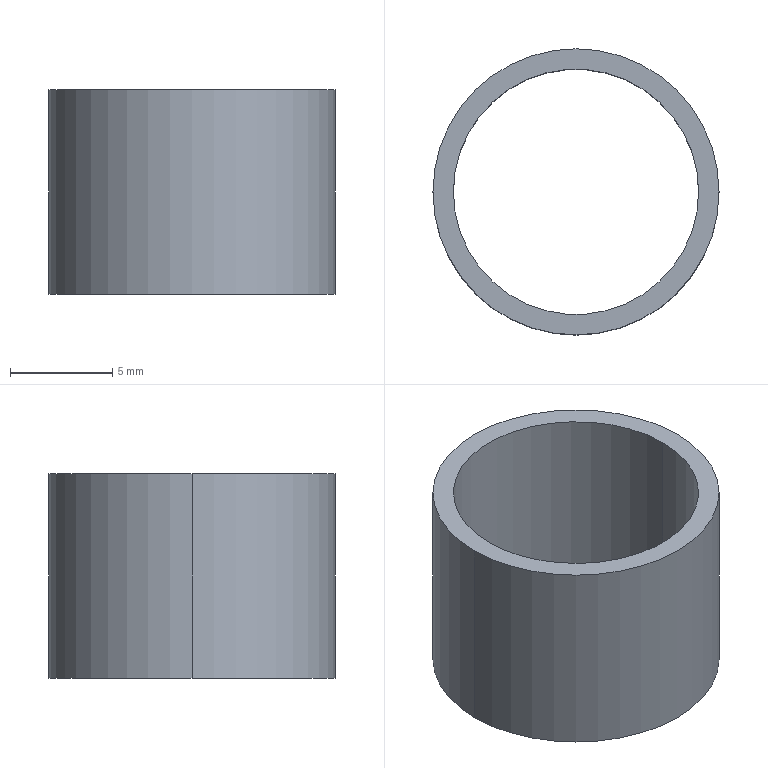Part | STEP file | steel sleeve 12-14-10 | 1 solid | 6 faces | box 14 x 14 x 10 mm | volume 408.407 mm3 | cylinder 4 | plane 2 | commonest cylinder face diameters 12 x2 14 x2
STEP:
#1=CARTESIAN_POINT('',(0.,0.,0.));
#2=DIRECTION('',(0.,0.,1.));
#3=DIRECTION('',(1.,0.,0.));
#4=AXIS2_PLACEMENT_3D('',#1,#2,#3);
#5=CARTESIAN_POINT('',(-6.,0.,10.));
#6=VERTEX_POINT('',#5);
#7=CARTESIAN_POINT('',(-6.,0.,0.));
#8=VERTEX_POINT('',#7);
#9=CARTESIAN_POINT('',(-6.,0.,10.));
#10=DIRECTION('',(0.,0.,-1.));
#11=VECTOR('',#10,1.);
#12=LINE('',#9,#11);
#13=CARTESIAN_POINT('',(0.,0.,10.));
#14=DIRECTION('',(0.,0.,-1.));
#15=DIRECTION('',(-1.,0.,0.));
#16=AXIS2_PLACEMENT_3D('',#13,#14,#15);
#17=CYLINDRICAL_SURFACE('',#16,6.);
#18=CARTESIAN_POINT('',(6.283,0.));
#19=DIRECTION('',(0.,1.));
#20=VECTOR('',#19,1.);
#21=LINE('',#18,#20);
#22=(GEOMETRIC_REPRESENTATION_CONTEXT(2)PARAMETRIC_REPRESENTATION_CONTEXT()REPRESENTATION_CONTEXT('',''));
#23=DEFINITIONAL_REPRESENTATION('',(#21),#22);
#24=PCURVE('',#17,#23);
#25=CARTESIAN_POINT('',(0.,0.,10.));
#26=DIRECTION('',(0.,0.,-1.));
#27=DIRECTION('',(-1.,0.,0.));
#28=AXIS2_PLACEMENT_3D('',#25,#26,#27);
#29=CYLINDRICAL_SURFACE('',#28,6.);
#30=CARTESIAN_POINT('',(0.,0.));
#31=DIRECTION('',(0.,1.));
#32=VECTOR('',#31,1.);
#33=LINE('',#30,#32);
#34=(GEOMETRIC_REPRESENTATION_CONTEXT(2)PARAMETRIC_REPRESENTATION_CONTEXT()REPRESENTATION_CONTEXT('',''));
#35=DEFINITIONAL_REPRESENTATION('',(#33),#34);
#36=PCURVE('',#29,#35);
#37=SURFACE_CURVE('',#12,(#24,#36),.PCURVE_S1.);
#38=EDGE_CURVE('',#6,#8,#37,.T.);
#39=ORIENTED_EDGE('',*,*,#38,.T.);
#40=CARTESIAN_POINT('',(6.,0.,0.));
#41=VERTEX_POINT('',#40);
#42=CARTESIAN_POINT('',(0.,0.,0.));
#43=DIRECTION('',(0.,0.,1.));
#44=DIRECTION('',(1.,0.,0.));
#45=AXIS2_PLACEMENT_3D('',#42,#43,#44);
#46=CIRCLE('',#45,6.);
#47=CARTESIAN_POINT('',(9.425,10.));
#48=DIRECTION('',(-1.,0.));
#49=VECTOR('',#48,1.);
#50=LINE('',#47,#49);
#51=(GEOMETRIC_REPRESENTATION_CONTEXT(2)PARAMETRIC_REPRESENTATION_CONTEXT()REPRESENTATION_CONTEXT('',''));
#52=DEFINITIONAL_REPRESENTATION('',(#50),#51);
#53=PCURVE('',#17,#52);
#54=CARTESIAN_POINT('',(0.,0.,0.));
#55=DIRECTION('',(0.,0.,1.));
#56=DIRECTION('',(1.,0.,0.));
#57=AXIS2_PLACEMENT_3D('',#54,#55,#56);
#58=PLANE('',#57);
#59=CARTESIAN_POINT('',(0.,0.));
#60=DIRECTION('',(1.,0.));
#61=AXIS2_PLACEMENT_2D('',#59,#60);
#62=CIRCLE('',#61,6.);
#63=(GEOMETRIC_REPRESENTATION_CONTEXT(2)PARAMETRIC_REPRESENTATION_CONTEXT()REPRESENTATION_CONTEXT('',''));
#64=DEFINITIONAL_REPRESENTATION('',(#62),#63);
#65=PCURVE('',#58,#64);
#66=SURFACE_CURVE('',#46,(#53,#65),.PCURVE_S1.);
#67=EDGE_CURVE('',#8,#41,#66,.T.);
#68=ORIENTED_EDGE('',*,*,#67,.T.);
#69=CARTESIAN_POINT('',(6.,0.,10.));
#70=VERTEX_POINT('',#69);
#71=CARTESIAN_POINT('',(6.,0.,10.));
#72=DIRECTION('',(0.,0.,-1.));
#73=VECTOR('',#72,1.);
#74=LINE('',#71,#73);
#75=CARTESIAN_POINT('',(3.142,0.));
#76=DIRECTION('',(0.,1.));
#77=VECTOR('',#76,1.);
#78=LINE('',#75,#77);
#79=(GEOMETRIC_REPRESENTATION_CONTEXT(2)PARAMETRIC_REPRESENTATION_CONTEXT()REPRESENTATION_CONTEXT('',''));
#80=DEFINITIONAL_REPRESENTATION('',(#78),#79);
#81=PCURVE('',#17,#80);
#82=CARTESIAN_POINT('',(3.142,0.));
#83=DIRECTION('',(0.,1.));
#84=VECTOR('',#83,1.);
#85=LINE('',#82,#84);
#86=(GEOMETRIC_REPRESENTATION_CONTEXT(2)PARAMETRIC_REPRESENTATION_CONTEXT()REPRESENTATION_CONTEXT('',''));
#87=DEFINITIONAL_REPRESENTATION('',(#85),#86);
#88=PCURVE('',#29,#87);
#89=SURFACE_CURVE('',#74,(#81,#88),.PCURVE_S1.);
#90=EDGE_CURVE('',#70,#41,#89,.T.);
#91=ORIENTED_EDGE('',*,*,#90,.F.);
#92=CARTESIAN_POINT('',(0.,0.,10.));
#93=DIRECTION('',(0.,0.,1.));
#94=DIRECTION('',(1.,0.,0.));
#95=AXIS2_PLACEMENT_3D('',#92,#93,#94);
#96=CIRCLE('',#95,6.);
#97=CARTESIAN_POINT('',(9.425,0.));
#98=DIRECTION('',(-1.,0.));
#99=VECTOR('',#98,1.);
#100=LINE('',#97,#99);
#101=(GEOMETRIC_REPRESENTATION_CONTEXT(2)PARAMETRIC_REPRESENTATION_CONTEXT()REPRESENTATION_CONTEXT('',''));
#102=DEFINITIONAL_REPRESENTATION('',(#100),#101);
#103=PCURVE('',#17,#102);
#104=CARTESIAN_POINT('',(0.,0.,10.));
#105=DIRECTION('',(0.,0.,1.));
#106=DIRECTION('',(1.,0.,0.));
#107=AXIS2_PLACEMENT_3D('',#104,#105,#106);
#108=PLANE('',#107);
#109=CARTESIAN_POINT('',(0.,0.));
#110=DIRECTION('',(1.,0.));
#111=AXIS2_PLACEMENT_2D('',#109,#110);
#112=CIRCLE('',#111,6.);
#113=(GEOMETRIC_REPRESENTATION_CONTEXT(2)PARAMETRIC_REPRESENTATION_CONTEXT()REPRESENTATION_CONTEXT('',''));
#114=DEFINITIONAL_REPRESENTATION('',(#112),#113);
#115=PCURVE('',#108,#114);
#116=SURFACE_CURVE('',#96,(#103,#115),.PCURVE_S1.);
#117=EDGE_CURVE('',#6,#70,#116,.T.);
#118=ORIENTED_EDGE('',*,*,#117,.F.);
#119=EDGE_LOOP('',(#39,#68,#91,#118));
#120=FACE_BOUND('',#119,.F.);
#121=ADVANCED_FACE('',(#120),#17,.F.);
#122=CARTESIAN_POINT('',(7.,0.,10.));
#123=VERTEX_POINT('',#122);
#124=CARTESIAN_POINT('',(-7.,0.,10.));
#125=VERTEX_POINT('',#124);
#126=CARTESIAN_POINT('',(0.,0.,10.));
#127=DIRECTION('',(0.,0.,1.));
#128=DIRECTION('',(1.,0.,0.));
#129=AXIS2_PLACEMENT_3D('',#126,#127,#128);
#130=CIRCLE('',#129,7.);
#131=CARTESIAN_POINT('',(0.,0.,10.));
#132=DIRECTION('',(0.,0.,-1.));
#133=DIRECTION('',(-1.,0.,0.));
#134=AXIS2_PLACEMENT_3D('',#131,#132,#133);
#135=CYLINDRICAL_SURFACE('',#134,7.);
#136=CARTESIAN_POINT('',(3.142,0.));
#137=DIRECTION('',(-1.,0.));
#138=VECTOR('',#137,1.);
#139=LINE('',#136,#138);
#140=(GEOMETRIC_REPRESENTATION_CONTEXT(2)PARAMETRIC_REPRESENTATION_CONTEXT()REPRESENTATION_CONTEXT('',''));
#141=DEFINITIONAL_REPRESENTATION('',(#139),#140);
#142=PCURVE('',#135,#141);
#143=CARTESIAN_POINT('',(0.,0.));
#144=DIRECTION('',(1.,0.));
#145=AXIS2_PLACEMENT_2D('',#143,#144);
#146=CIRCLE('',#145,7.);
#147=(GEOMETRIC_REPRESENTATION_CONTEXT(2)PARAMETRIC_REPRESENTATION_CONTEXT()REPRESENTATION_CONTEXT('',''));
#148=DEFINITIONAL_REPRESENTATION('',(#146),#147);
#149=PCURVE('',#108,#148);
#150=SURFACE_CURVE('',#130,(#142,#149),.PCURVE_S1.);
#151=EDGE_CURVE('',#123,#125,#150,.T.);
#152=ORIENTED_EDGE('',*,*,#151,.F.);
#153=CARTESIAN_POINT('',(7.,0.,0.));
#154=VERTEX_POINT('',#153);
#155=CARTESIAN_POINT('',(7.,0.,10.));
#156=DIRECTION('',(0.,0.,-1.));
#157=VECTOR('',#156,1.);
#158=LINE('',#155,#157);
#159=CARTESIAN_POINT('',(3.142,0.));
#160=DIRECTION('',(0.,1.));
#161=VECTOR('',#160,1.);
#162=LINE('',#159,#161);
#163=(GEOMETRIC_REPRESENTATION_CONTEXT(2)PARAMETRIC_REPRESENTATION_CONTEXT()REPRESENTATION_CONTEXT('',''));
#164=DEFINITIONAL_REPRESENTATION('',(#162),#163);
#165=PCURVE('',#135,#164);
#166=CARTESIAN_POINT('',(0.,0.,10.));
#167=DIRECTION('',(0.,0.,-1.));
#168=DIRECTION('',(-1.,0.,0.));
#169=AXIS2_PLACEMENT_3D('',#166,#167,#168);
#170=CYLINDRICAL_SURFACE('',#169,7.);
#171=CARTESIAN_POINT('',(3.142,0.));
#172=DIRECTION('',(0.,1.));
#173=VECTOR('',#172,1.);
#174=LINE('',#171,#173);
#175=(GEOMETRIC_REPRESENTATION_CONTEXT(2)PARAMETRIC_REPRESENTATION_CONTEXT()REPRESENTATION_CONTEXT('',''));
#176=DEFINITIONAL_REPRESENTATION('',(#174),#175);
#177=PCURVE('',#170,#176);
#178=SURFACE_CURVE('',#158,(#165,#177),.PCURVE_S1.);
#179=EDGE_CURVE('',#123,#154,#178,.T.);
#180=ORIENTED_EDGE('',*,*,#179,.T.);
#181=CARTESIAN_POINT('',(-7.,0.,0.));
#182=VERTEX_POINT('',#181);
#183=CARTESIAN_POINT('',(0.,0.,0.));
#184=DIRECTION('',(0.,0.,1.));
#185=DIRECTION('',(1.,0.,0.));
#186=AXIS2_PLACEMENT_3D('',#183,#184,#185);
#187=CIRCLE('',#186,7.);
#188=CARTESIAN_POINT('',(3.142,10.));
#189=DIRECTION('',(-1.,0.));
#190=VECTOR('',#189,1.);
#191=LINE('',#188,#190);
#192=(GEOMETRIC_REPRESENTATION_CONTEXT(2)PARAMETRIC_REPRESENTATION_CONTEXT()REPRESENTATION_CONTEXT('',''));
#193=DEFINITIONAL_REPRESENTATION('',(#191),#192);
#194=PCURVE('',#135,#193);
#195=CARTESIAN_POINT('',(0.,0.));
#196=DIRECTION('',(1.,0.));
#197=AXIS2_PLACEMENT_2D('',#195,#196);
#198=CIRCLE('',#197,7.);
#199=(GEOMETRIC_REPRESENTATION_CONTEXT(2)PARAMETRIC_REPRESENTATION_CONTEXT()REPRESENTATION_CONTEXT('',''));
#200=DEFINITIONAL_REPRESENTATION('',(#198),#199);
#201=PCURVE('',#58,#200);
#202=SURFACE_CURVE('',#187,(#194,#201),.PCURVE_S1.);
#203=EDGE_CURVE('',#154,#182,#202,.T.);
#204=ORIENTED_EDGE('',*,*,#203,.T.);
#205=CARTESIAN_POINT('',(-7.,0.,10.));
#206=DIRECTION('',(0.,0.,-1.));
#207=VECTOR('',#206,1.);
#208=LINE('',#205,#207);
#209=CARTESIAN_POINT('',(0.,0.));
#210=DIRECTION('',(0.,1.));
#211=VECTOR('',#210,1.);
#212=LINE('',#209,#211);
#213=(GEOMETRIC_REPRESENTATION_CONTEXT(2)PARAMETRIC_REPRESENTATION_CONTEXT()REPRESENTATION_CONTEXT('',''));
#214=DEFINITIONAL_REPRESENTATION('',(#212),#213);
#215=PCURVE('',#135,#214);
#216=CARTESIAN_POINT('',(6.283,0.));
#217=DIRECTION('',(0.,1.));
#218=VECTOR('',#217,1.);
#219=LINE('',#216,#218);
#220=(GEOMETRIC_REPRESENTATION_CONTEXT(2)PARAMETRIC_REPRESENTATION_CONTEXT()REPRESENTATION_CONTEXT('',''));
#221=DEFINITIONAL_REPRESENTATION('',(#219),#220);
#222=PCURVE('',#170,#221);
#223=SURFACE_CURVE('',#208,(#215,#222),.PCURVE_S1.);
#224=EDGE_CURVE('',#125,#182,#223,.T.);
#225=ORIENTED_EDGE('',*,*,#224,.F.);
#226=EDGE_LOOP('',(#152,#180,#204,#225));
#227=FACE_BOUND('',#226,.T.);
#228=ADVANCED_FACE('',(#227),#135,.T.);
#229=CARTESIAN_POINT('',(0.,0.,10.));
#230=DIRECTION('',(0.,0.,1.));
#231=DIRECTION('',(1.,0.,0.));
#232=AXIS2_PLACEMENT_3D('',#229,#230,#231);
#233=CIRCLE('',#232,7.);
#234=CARTESIAN_POINT('',(0.,0.));
#235=DIRECTION('',(1.,0.));
#236=AXIS2_PLACEMENT_2D('',#234,#235);
#237=CIRCLE('',#236,7.);
#238=(GEOMETRIC_REPRESENTATION_CONTEXT(2)PARAMETRIC_REPRESENTATION_CONTEXT()REPRESENTATION_CONTEXT('',''));
#239=DEFINITIONAL_REPRESENTATION('',(#237),#238);
#240=PCURVE('',#108,#239);
#241=CARTESIAN_POINT('',(9.425,0.));
#242=DIRECTION('',(-1.,0.));
#243=VECTOR('',#242,1.);
#244=LINE('',#241,#243);
#245=(GEOMETRIC_REPRESENTATION_CONTEXT(2)PARAMETRIC_REPRESENTATION_CONTEXT()REPRESENTATION_CONTEXT('',''));
#246=DEFINITIONAL_REPRESENTATION('',(#244),#245);
#247=PCURVE('',#170,#246);
#248=SURFACE_CURVE('',#233,(#240,#247),.PCURVE_S1.);
#249=EDGE_CURVE('',#125,#123,#248,.T.);
#250=ORIENTED_EDGE('',*,*,#249,.T.);
#251=ORIENTED_EDGE('',*,*,#151,.T.);
#252=EDGE_LOOP('',(#250,#251));
#253=FACE_BOUND('',#252,.T.);
#254=ORIENTED_EDGE('',*,*,#117,.F.);
#255=CARTESIAN_POINT('',(0.,0.,10.));
#256=DIRECTION('',(0.,0.,1.));
#257=DIRECTION('',(1.,0.,0.));
#258=AXIS2_PLACEMENT_3D('',#255,#256,#257);
#259=CIRCLE('',#258,6.);
#260=CARTESIAN_POINT('',(0.,0.));
#261=DIRECTION('',(1.,0.));
#262=AXIS2_PLACEMENT_2D('',#260,#261);
#263=CIRCLE('',#262,6.);
#264=(GEOMETRIC_REPRESENTATION_CONTEXT(2)PARAMETRIC_REPRESENTATION_CONTEXT()REPRESENTATION_CONTEXT('',''));
#265=DEFINITIONAL_REPRESENTATION('',(#263),#264);
#266=PCURVE('',#108,#265);
#267=CARTESIAN_POINT('',(3.142,0.));
#268=DIRECTION('',(-1.,0.));
#269=VECTOR('',#268,1.);
#270=LINE('',#267,#269);
#271=(GEOMETRIC_REPRESENTATION_CONTEXT(2)PARAMETRIC_REPRESENTATION_CONTEXT()REPRESENTATION_CONTEXT('',''));
#272=DEFINITIONAL_REPRESENTATION('',(#270),#271);
#273=PCURVE('',#29,#272);
#274=SURFACE_CURVE('',#259,(#266,#273),.PCURVE_S1.);
#275=EDGE_CURVE('',#70,#6,#274,.T.);
#276=ORIENTED_EDGE('',*,*,#275,.F.);
#277=EDGE_LOOP('',(#254,#276));
#278=FACE_BOUND('',#277,.T.);
#279=ADVANCED_FACE('',(#253,#278),#108,.T.);
#280=CARTESIAN_POINT('',(0.,0.,0.));
#281=DIRECTION('',(0.,0.,1.));
#282=DIRECTION('',(1.,0.,0.));
#283=AXIS2_PLACEMENT_3D('',#280,#281,#282);
#284=CIRCLE('',#283,7.);
#285=CARTESIAN_POINT('',(0.,0.));
#286=DIRECTION('',(1.,0.));
#287=AXIS2_PLACEMENT_2D('',#285,#286);
#288=CIRCLE('',#287,7.);
#289=(GEOMETRIC_REPRESENTATION_CONTEXT(2)PARAMETRIC_REPRESENTATION_CONTEXT()REPRESENTATION_CONTEXT('',''));
#290=DEFINITIONAL_REPRESENTATION('',(#288),#289);
#291=PCURVE('',#58,#290);
#292=CARTESIAN_POINT('',(9.425,10.));
#293=DIRECTION('',(-1.,0.));
#294=VECTOR('',#293,1.);
#295=LINE('',#292,#294);
#296=(GEOMETRIC_REPRESENTATION_CONTEXT(2)PARAMETRIC_REPRESENTATION_CONTEXT()REPRESENTATION_CONTEXT('',''));
#297=DEFINITIONAL_REPRESENTATION('',(#295),#296);
#298=PCURVE('',#170,#297);
#299=SURFACE_CURVE('',#284,(#291,#298),.PCURVE_S1.);
#300=EDGE_CURVE('',#182,#154,#299,.T.);
#301=ORIENTED_EDGE('',*,*,#300,.F.);
#302=ORIENTED_EDGE('',*,*,#203,.F.);
#303=EDGE_LOOP('',(#301,#302));
#304=FACE_BOUND('',#303,.T.);
#305=ORIENTED_EDGE('',*,*,#67,.T.);
#306=CARTESIAN_POINT('',(0.,0.,0.));
#307=DIRECTION('',(0.,0.,1.));
#308=DIRECTION('',(1.,0.,0.));
#309=AXIS2_PLACEMENT_3D('',#306,#307,#308);
#310=CIRCLE('',#309,6.);
#311=CARTESIAN_POINT('',(0.,0.));
#312=DIRECTION('',(1.,0.));
#313=AXIS2_PLACEMENT_2D('',#311,#312);
#314=CIRCLE('',#313,6.);
#315=(GEOMETRIC_REPRESENTATION_CONTEXT(2)PARAMETRIC_REPRESENTATION_CONTEXT()REPRESENTATION_CONTEXT('',''));
#316=DEFINITIONAL_REPRESENTATION('',(#314),#315);
#317=PCURVE('',#58,#316);
#318=CARTESIAN_POINT('',(3.142,10.));
#319=DIRECTION('',(-1.,0.));
#320=VECTOR('',#319,1.);
#321=LINE('',#318,#320);
#322=(GEOMETRIC_REPRESENTATION_CONTEXT(2)PARAMETRIC_REPRESENTATION_CONTEXT()REPRESENTATION_CONTEXT('',''));
#323=DEFINITIONAL_REPRESENTATION('',(#321),#322);
#324=PCURVE('',#29,#323);
#325=SURFACE_CURVE('',#310,(#317,#324),.PCURVE_S1.);
#326=EDGE_CURVE('',#41,#8,#325,.T.);
#327=ORIENTED_EDGE('',*,*,#326,.T.);
#328=EDGE_LOOP('',(#305,#327));
#329=FACE_BOUND('',#328,.T.);
#330=ADVANCED_FACE('',(#304,#329),#58,.F.);
#331=ORIENTED_EDGE('',*,*,#179,.F.);
#332=ORIENTED_EDGE('',*,*,#249,.F.);
#333=ORIENTED_EDGE('',*,*,#224,.T.);
#334=ORIENTED_EDGE('',*,*,#300,.T.);
#335=EDGE_LOOP('',(#331,#332,#333,#334));
#336=FACE_BOUND('',#335,.T.);
#337=ADVANCED_FACE('',(#336),#170,.T.);
#338=ORIENTED_EDGE('',*,*,#326,.T.);
#339=ORIENTED_EDGE('',*,*,#38,.F.);
#340=ORIENTED_EDGE('',*,*,#275,.F.);
#341=ORIENTED_EDGE('',*,*,#90,.T.);
#342=EDGE_LOOP('',(#338,#339,#340,#341));
#343=FACE_BOUND('',#342,.F.);
#344=ADVANCED_FACE('',(#343),#29,.F.);
#345=CLOSED_SHELL('',(#121,#228,#279,#330,#337,#344));
#346=MANIFOLD_SOLID_BREP('',#345);
#347=(LENGTH_UNIT()NAMED_UNIT(*)SI_UNIT(.MILLI.,.METRE.));
#348=UNCERTAINTY_MEASURE_WITH_UNIT(LENGTH_MEASURE(0.0000001),#347,'','');
#349=(NAMED_UNIT(*)PLANE_ANGLE_UNIT()SI_UNIT($,.RADIAN.));
#350=(NAMED_UNIT(*)SI_UNIT($,.STERADIAN.)SOLID_ANGLE_UNIT());
#351=(GEOMETRIC_REPRESENTATION_CONTEXT(3)GLOBAL_UNCERTAINTY_ASSIGNED_CONTEXT((#348))GLOBAL_UNIT_ASSIGNED_CONTEXT((#347,#349,#350))REPRESENTATION_CONTEXT('',''));
#352=ADVANCED_BREP_SHAPE_REPRESENTATION('',(#4,#346),#351);